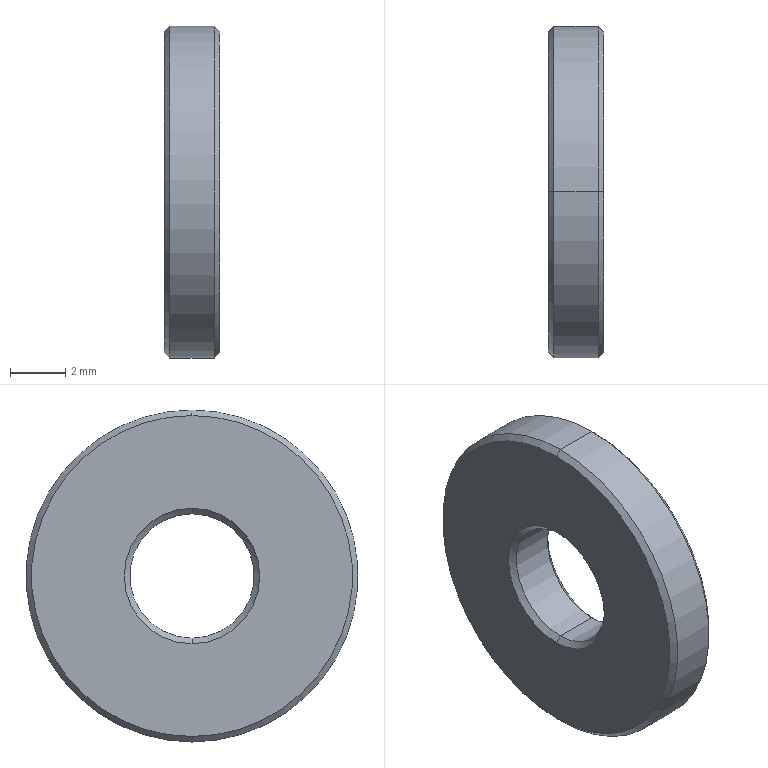Part | STEP file | 03-10 Bearing cover plate 2 | 1 solid | 14 faces | box 2 x 12 x 12 mm | volume 192.313 mm3 | cone 8 | cylinder 4 | plane 2 | commonest cylinder face diameters 4.5 x2 12 x2
STEP:
#1=CARTESIAN_POINT('',(0.,0.,0.));
#2=DIRECTION('',(0.,0.,1.));
#3=DIRECTION('',(1.,0.,0.));
#4=AXIS2_PLACEMENT_3D('',#1,#2,#3);
#5=CARTESIAN_POINT('',(1.8,0.,-2.25));
#6=VERTEX_POINT('',#5);
#7=CARTESIAN_POINT('',(2.,0.,-2.45));
#8=VERTEX_POINT('',#7);
#9=CARTESIAN_POINT('',(1.8,0.,-2.25));
#10=DIRECTION('',(0.7071,0.,-0.7071));
#11=VECTOR('',#10,1.);
#12=LINE('',#9,#11);
#13=CARTESIAN_POINT('',(1.8,0.,0.));
#14=DIRECTION('',(1.,0.,0.));
#15=DIRECTION('',(0.,0.,-1.));
#16=AXIS2_PLACEMENT_3D('',#13,#14,#15);
#17=CONICAL_SURFACE('',#16,2.25,0.7854);
#18=CARTESIAN_POINT('',(6.283,0.));
#19=DIRECTION('',(0.,1.));
#20=VECTOR('',#19,1.);
#21=LINE('',#18,#20);
#22=(GEOMETRIC_REPRESENTATION_CONTEXT(2)PARAMETRIC_REPRESENTATION_CONTEXT()REPRESENTATION_CONTEXT('',''));
#23=DEFINITIONAL_REPRESENTATION('',(#21),#22);
#24=PCURVE('',#17,#23);
#25=CARTESIAN_POINT('',(1.8,0.,0.));
#26=DIRECTION('',(1.,0.,0.));
#27=DIRECTION('',(0.,0.,-1.));
#28=AXIS2_PLACEMENT_3D('',#25,#26,#27);
#29=CONICAL_SURFACE('',#28,2.25,0.7854);
#30=CARTESIAN_POINT('',(0.,0.));
#31=DIRECTION('',(0.,1.));
#32=VECTOR('',#31,1.);
#33=LINE('',#30,#32);
#34=(GEOMETRIC_REPRESENTATION_CONTEXT(2)PARAMETRIC_REPRESENTATION_CONTEXT()REPRESENTATION_CONTEXT('',''));
#35=DEFINITIONAL_REPRESENTATION('',(#33),#34);
#36=PCURVE('',#29,#35);
#37=SURFACE_CURVE('',#12,(#24,#36),.PCURVE_S1.);
#38=EDGE_CURVE('',#6,#8,#37,.T.);
#39=ORIENTED_EDGE('',*,*,#38,.T.);
#40=CARTESIAN_POINT('',(2.,0.,2.45));
#41=VERTEX_POINT('',#40);
#42=CARTESIAN_POINT('',(2.,0.,0.));
#43=DIRECTION('',(1.,0.,0.));
#44=DIRECTION('',(0.,0.,-1.));
#45=AXIS2_PLACEMENT_3D('',#42,#43,#44);
#46=CIRCLE('',#45,2.45);
#47=CARTESIAN_POINT('',(0.,0.2));
#48=DIRECTION('',(1.,0.));
#49=VECTOR('',#48,1.);
#50=LINE('',#47,#49);
#51=(GEOMETRIC_REPRESENTATION_CONTEXT(2)PARAMETRIC_REPRESENTATION_CONTEXT()REPRESENTATION_CONTEXT('',''));
#52=DEFINITIONAL_REPRESENTATION('',(#50),#51);
#53=PCURVE('',#17,#52);
#54=CARTESIAN_POINT('',(2.,-5.87,5.87));
#55=DIRECTION('',(1.,0.,0.));
#56=DIRECTION('',(0.,0.,-1.));
#57=AXIS2_PLACEMENT_3D('',#54,#55,#56);
#58=PLANE('',#57);
#59=CARTESIAN_POINT('',(5.87,5.87));
#60=DIRECTION('',(1.,0.));
#61=AXIS2_PLACEMENT_2D('',#59,#60);
#62=CIRCLE('',#61,2.45);
#63=(GEOMETRIC_REPRESENTATION_CONTEXT(2)PARAMETRIC_REPRESENTATION_CONTEXT()REPRESENTATION_CONTEXT('',''));
#64=DEFINITIONAL_REPRESENTATION('',(#62),#63);
#65=PCURVE('',#58,#64);
#66=SURFACE_CURVE('',#46,(#53,#65),.PCURVE_S1.);
#67=EDGE_CURVE('',#41,#8,#66,.T.);
#68=ORIENTED_EDGE('',*,*,#67,.F.);
#69=CARTESIAN_POINT('',(1.8,0.,2.25));
#70=VERTEX_POINT('',#69);
#71=CARTESIAN_POINT('',(1.8,0.,2.25));
#72=DIRECTION('',(0.7071,0.,0.7071));
#73=VECTOR('',#72,1.);
#74=LINE('',#71,#73);
#75=CARTESIAN_POINT('',(3.142,0.));
#76=DIRECTION('',(0.,1.));
#77=VECTOR('',#76,1.);
#78=LINE('',#75,#77);
#79=(GEOMETRIC_REPRESENTATION_CONTEXT(2)PARAMETRIC_REPRESENTATION_CONTEXT()REPRESENTATION_CONTEXT('',''));
#80=DEFINITIONAL_REPRESENTATION('',(#78),#79);
#81=PCURVE('',#17,#80);
#82=CARTESIAN_POINT('',(3.142,0.));
#83=DIRECTION('',(0.,1.));
#84=VECTOR('',#83,1.);
#85=LINE('',#82,#84);
#86=(GEOMETRIC_REPRESENTATION_CONTEXT(2)PARAMETRIC_REPRESENTATION_CONTEXT()REPRESENTATION_CONTEXT('',''));
#87=DEFINITIONAL_REPRESENTATION('',(#85),#86);
#88=PCURVE('',#29,#87);
#89=SURFACE_CURVE('',#74,(#81,#88),.PCURVE_S1.);
#90=EDGE_CURVE('',#70,#41,#89,.T.);
#91=ORIENTED_EDGE('',*,*,#90,.F.);
#92=CARTESIAN_POINT('',(1.8,0.,0.));
#93=DIRECTION('',(-1.,0.,0.));
#94=DIRECTION('',(0.,0.,-1.));
#95=AXIS2_PLACEMENT_3D('',#92,#93,#94);
#96=CIRCLE('',#95,2.25);
#97=CARTESIAN_POINT('',(6.283,0.));
#98=DIRECTION('',(-1.,0.));
#99=VECTOR('',#98,1.);
#100=LINE('',#97,#99);
#101=(GEOMETRIC_REPRESENTATION_CONTEXT(2)PARAMETRIC_REPRESENTATION_CONTEXT()REPRESENTATION_CONTEXT('',''));
#102=DEFINITIONAL_REPRESENTATION('',(#100),#101);
#103=PCURVE('',#17,#102);
#104=CARTESIAN_POINT('',(1.8,0.,0.));
#105=DIRECTION('',(-1.,0.,0.));
#106=DIRECTION('',(0.,0.,1.));
#107=AXIS2_PLACEMENT_3D('',#104,#105,#106);
#108=CYLINDRICAL_SURFACE('',#107,2.25);
#109=CARTESIAN_POINT('',(3.142,0.));
#110=DIRECTION('',(1.,0.));
#111=VECTOR('',#110,1.);
#112=LINE('',#109,#111);
#113=(GEOMETRIC_REPRESENTATION_CONTEXT(2)PARAMETRIC_REPRESENTATION_CONTEXT()REPRESENTATION_CONTEXT('',''));
#114=DEFINITIONAL_REPRESENTATION('',(#112),#113);
#115=PCURVE('',#108,#114);
#116=SURFACE_CURVE('',#96,(#103,#115),.PCURVE_S1.);
#117=EDGE_CURVE('',#6,#70,#116,.T.);
#118=ORIENTED_EDGE('',*,*,#117,.F.);
#119=EDGE_LOOP('',(#39,#68,#91,#118));
#120=FACE_BOUND('',#119,.F.);
#121=ADVANCED_FACE('',(#120),#17,.F.);
#122=CARTESIAN_POINT('',(0.2,0.,2.25));
#123=VERTEX_POINT('',#122);
#124=CARTESIAN_POINT('',(1.8,0.,2.25));
#125=DIRECTION('',(-1.,0.,0.));
#126=VECTOR('',#125,1.);
#127=LINE('',#124,#126);
#128=CARTESIAN_POINT('',(6.283,0.));
#129=DIRECTION('',(0.,1.));
#130=VECTOR('',#129,1.);
#131=LINE('',#128,#130);
#132=(GEOMETRIC_REPRESENTATION_CONTEXT(2)PARAMETRIC_REPRESENTATION_CONTEXT()REPRESENTATION_CONTEXT('',''));
#133=DEFINITIONAL_REPRESENTATION('',(#131),#132);
#134=PCURVE('',#108,#133);
#135=CARTESIAN_POINT('',(1.8,0.,0.));
#136=DIRECTION('',(-1.,0.,0.));
#137=DIRECTION('',(0.,0.,1.));
#138=AXIS2_PLACEMENT_3D('',#135,#136,#137);
#139=CYLINDRICAL_SURFACE('',#138,2.25);
#140=CARTESIAN_POINT('',(0.,0.));
#141=DIRECTION('',(0.,1.));
#142=VECTOR('',#141,1.);
#143=LINE('',#140,#142);
#144=(GEOMETRIC_REPRESENTATION_CONTEXT(2)PARAMETRIC_REPRESENTATION_CONTEXT()REPRESENTATION_CONTEXT('',''));
#145=DEFINITIONAL_REPRESENTATION('',(#143),#144);
#146=PCURVE('',#139,#145);
#147=SURFACE_CURVE('',#127,(#134,#146),.PCURVE_S1.);
#148=EDGE_CURVE('',#70,#123,#147,.T.);
#149=ORIENTED_EDGE('',*,*,#148,.T.);
#150=CARTESIAN_POINT('',(0.2,0.,-2.25));
#151=VERTEX_POINT('',#150);
#152=CARTESIAN_POINT('',(0.2,0.,0.));
#153=DIRECTION('',(-1.,0.,0.));
#154=DIRECTION('',(0.,0.,1.));
#155=AXIS2_PLACEMENT_3D('',#152,#153,#154);
#156=CIRCLE('',#155,2.25);
#157=CARTESIAN_POINT('',(0.,1.6));
#158=DIRECTION('',(1.,0.));
#159=VECTOR('',#158,1.);
#160=LINE('',#157,#159);
#161=(GEOMETRIC_REPRESENTATION_CONTEXT(2)PARAMETRIC_REPRESENTATION_CONTEXT()REPRESENTATION_CONTEXT('',''));
#162=DEFINITIONAL_REPRESENTATION('',(#160),#161);
#163=PCURVE('',#108,#162);
#164=CARTESIAN_POINT('',(0.2,0.,0.));
#165=DIRECTION('',(-1.,0.,0.));
#166=DIRECTION('',(0.,0.,1.));
#167=AXIS2_PLACEMENT_3D('',#164,#165,#166);
#168=CONICAL_SURFACE('',#167,2.25,0.7854);
#169=CARTESIAN_POINT('',(0.,0.));
#170=DIRECTION('',(1.,0.));
#171=VECTOR('',#170,1.);
#172=LINE('',#169,#171);
#173=(GEOMETRIC_REPRESENTATION_CONTEXT(2)PARAMETRIC_REPRESENTATION_CONTEXT()REPRESENTATION_CONTEXT('',''));
#174=DEFINITIONAL_REPRESENTATION('',(#172),#173);
#175=PCURVE('',#168,#174);
#176=SURFACE_CURVE('',#156,(#163,#175),.PCURVE_S1.);
#177=EDGE_CURVE('',#151,#123,#176,.T.);
#178=ORIENTED_EDGE('',*,*,#177,.F.);
#179=CARTESIAN_POINT('',(1.8,0.,-2.25));
#180=DIRECTION('',(-1.,0.,0.));
#181=VECTOR('',#180,1.);
#182=LINE('',#179,#181);
#183=CARTESIAN_POINT('',(3.142,0.));
#184=DIRECTION('',(0.,1.));
#185=VECTOR('',#184,1.);
#186=LINE('',#183,#185);
#187=(GEOMETRIC_REPRESENTATION_CONTEXT(2)PARAMETRIC_REPRESENTATION_CONTEXT()REPRESENTATION_CONTEXT('',''));
#188=DEFINITIONAL_REPRESENTATION('',(#186),#187);
#189=PCURVE('',#108,#188);
#190=CARTESIAN_POINT('',(3.142,0.));
#191=DIRECTION('',(0.,1.));
#192=VECTOR('',#191,1.);
#193=LINE('',#190,#192);
#194=(GEOMETRIC_REPRESENTATION_CONTEXT(2)PARAMETRIC_REPRESENTATION_CONTEXT()REPRESENTATION_CONTEXT('',''));
#195=DEFINITIONAL_REPRESENTATION('',(#193),#194);
#196=PCURVE('',#139,#195);
#197=SURFACE_CURVE('',#182,(#189,#196),.PCURVE_S1.);
#198=EDGE_CURVE('',#6,#151,#197,.T.);
#199=ORIENTED_EDGE('',*,*,#198,.F.);
#200=ORIENTED_EDGE('',*,*,#117,.T.);
#201=EDGE_LOOP('',(#149,#178,#199,#200));
#202=FACE_BOUND('',#201,.F.);
#203=ADVANCED_FACE('',(#202),#108,.F.);
#204=CARTESIAN_POINT('',(2.,0.,-5.8));
#205=VERTEX_POINT('',#204);
#206=CARTESIAN_POINT('',(2.,0.,5.8));
#207=VERTEX_POINT('',#206);
#208=CARTESIAN_POINT('',(2.,0.,0.));
#209=DIRECTION('',(1.,0.,0.));
#210=DIRECTION('',(0.,0.,1.));
#211=AXIS2_PLACEMENT_3D('',#208,#209,#210);
#212=CIRCLE('',#211,5.8);
#213=CARTESIAN_POINT('',(2.,0.,0.));
#214=DIRECTION('',(-1.,0.,0.));
#215=DIRECTION('',(0.,0.,1.));
#216=AXIS2_PLACEMENT_3D('',#213,#214,#215);
#217=CONICAL_SURFACE('',#216,5.8,0.7854);
#218=CARTESIAN_POINT('',(6.283,0.));
#219=DIRECTION('',(-1.,0.));
#220=VECTOR('',#219,1.);
#221=LINE('',#218,#220);
#222=(GEOMETRIC_REPRESENTATION_CONTEXT(2)PARAMETRIC_REPRESENTATION_CONTEXT()REPRESENTATION_CONTEXT('',''));
#223=DEFINITIONAL_REPRESENTATION('',(#221),#222);
#224=PCURVE('',#217,#223);
#225=CARTESIAN_POINT('',(5.87,5.87));
#226=DIRECTION('',(-1.,0.));
#227=AXIS2_PLACEMENT_2D('',#225,#226);
#228=CIRCLE('',#227,5.8);
#229=(GEOMETRIC_REPRESENTATION_CONTEXT(2)PARAMETRIC_REPRESENTATION_CONTEXT()REPRESENTATION_CONTEXT('',''));
#230=DEFINITIONAL_REPRESENTATION('',(#228),#229);
#231=PCURVE('',#58,#230);
#232=SURFACE_CURVE('',#212,(#224,#231),.PCURVE_S1.);
#233=EDGE_CURVE('',#205,#207,#232,.T.);
#234=ORIENTED_EDGE('',*,*,#233,.F.);
#235=CARTESIAN_POINT('',(1.8,0.,-6.));
#236=VERTEX_POINT('',#235);
#237=CARTESIAN_POINT('',(2.,0.,-5.8));
#238=DIRECTION('',(-0.7071,0.,-0.7071));
#239=VECTOR('',#238,1.);
#240=LINE('',#237,#239);
#241=CARTESIAN_POINT('',(3.142,0.));
#242=DIRECTION('',(0.,1.));
#243=VECTOR('',#242,1.);
#244=LINE('',#241,#243);
#245=(GEOMETRIC_REPRESENTATION_CONTEXT(2)PARAMETRIC_REPRESENTATION_CONTEXT()REPRESENTATION_CONTEXT('',''));
#246=DEFINITIONAL_REPRESENTATION('',(#244),#245);
#247=PCURVE('',#217,#246);
#248=CARTESIAN_POINT('',(2.,0.,0.));
#249=DIRECTION('',(-1.,0.,0.));
#250=DIRECTION('',(0.,0.,1.));
#251=AXIS2_PLACEMENT_3D('',#248,#249,#250);
#252=CONICAL_SURFACE('',#251,5.8,0.7854);
#253=CARTESIAN_POINT('',(3.142,0.));
#254=DIRECTION('',(0.,1.));
#255=VECTOR('',#254,1.);
#256=LINE('',#253,#255);
#257=(GEOMETRIC_REPRESENTATION_CONTEXT(2)PARAMETRIC_REPRESENTATION_CONTEXT()REPRESENTATION_CONTEXT('',''));
#258=DEFINITIONAL_REPRESENTATION('',(#256),#257);
#259=PCURVE('',#252,#258);
#260=SURFACE_CURVE('',#240,(#247,#259),.PCURVE_S1.);
#261=EDGE_CURVE('',#205,#236,#260,.T.);
#262=ORIENTED_EDGE('',*,*,#261,.T.);
#263=CARTESIAN_POINT('',(1.8,0.,6.));
#264=VERTEX_POINT('',#263);
#265=CARTESIAN_POINT('',(1.8,0.,0.));
#266=DIRECTION('',(-1.,0.,0.));
#267=DIRECTION('',(0.,0.,1.));
#268=AXIS2_PLACEMENT_3D('',#265,#266,#267);
#269=CIRCLE('',#268,6.);
#270=CARTESIAN_POINT('',(0.,0.2));
#271=DIRECTION('',(1.,0.));
#272=VECTOR('',#271,1.);
#273=LINE('',#270,#272);
#274=(GEOMETRIC_REPRESENTATION_CONTEXT(2)PARAMETRIC_REPRESENTATION_CONTEXT()REPRESENTATION_CONTEXT('',''));
#275=DEFINITIONAL_REPRESENTATION('',(#273),#274);
#276=PCURVE('',#217,#275);
#277=CARTESIAN_POINT('',(1.8,0.,0.));
#278=DIRECTION('',(-1.,0.,0.));
#279=DIRECTION('',(0.,0.,1.));
#280=AXIS2_PLACEMENT_3D('',#277,#278,#279);
#281=CYLINDRICAL_SURFACE('',#280,6.);
#282=CARTESIAN_POINT('',(0.,0.));
#283=DIRECTION('',(1.,0.));
#284=VECTOR('',#283,1.);
#285=LINE('',#282,#284);
#286=(GEOMETRIC_REPRESENTATION_CONTEXT(2)PARAMETRIC_REPRESENTATION_CONTEXT()REPRESENTATION_CONTEXT('',''));
#287=DEFINITIONAL_REPRESENTATION('',(#285),#286);
#288=PCURVE('',#281,#287);
#289=SURFACE_CURVE('',#269,(#276,#288),.PCURVE_S1.);
#290=EDGE_CURVE('',#264,#236,#289,.T.);
#291=ORIENTED_EDGE('',*,*,#290,.F.);
#292=CARTESIAN_POINT('',(2.,0.,5.8));
#293=DIRECTION('',(-0.7071,0.,0.7071));
#294=VECTOR('',#293,1.);
#295=LINE('',#292,#294);
#296=CARTESIAN_POINT('',(0.,0.));
#297=DIRECTION('',(0.,1.));
#298=VECTOR('',#297,1.);
#299=LINE('',#296,#298);
#300=(GEOMETRIC_REPRESENTATION_CONTEXT(2)PARAMETRIC_REPRESENTATION_CONTEXT()REPRESENTATION_CONTEXT('',''));
#301=DEFINITIONAL_REPRESENTATION('',(#299),#300);
#302=PCURVE('',#217,#301);
#303=CARTESIAN_POINT('',(6.283,0.));
#304=DIRECTION('',(0.,1.));
#305=VECTOR('',#304,1.);
#306=LINE('',#303,#305);
#307=(GEOMETRIC_REPRESENTATION_CONTEXT(2)PARAMETRIC_REPRESENTATION_CONTEXT()REPRESENTATION_CONTEXT('',''));
#308=DEFINITIONAL_REPRESENTATION('',(#306),#307);
#309=PCURVE('',#252,#308);
#310=SURFACE_CURVE('',#295,(#302,#309),.PCURVE_S1.);
#311=EDGE_CURVE('',#207,#264,#310,.T.);
#312=ORIENTED_EDGE('',*,*,#311,.F.);
#313=EDGE_LOOP('',(#234,#262,#291,#312));
#314=FACE_BOUND('',#313,.T.);
#315=ADVANCED_FACE('',(#314),#217,.T.);
#316=CARTESIAN_POINT('',(0.,0.,2.45));
#317=VERTEX_POINT('',#316);
#318=CARTESIAN_POINT('',(0.2,0.,2.25));
#319=DIRECTION('',(-0.7071,0.,0.7071));
#320=VECTOR('',#319,1.);
#321=LINE('',#318,#320);
#322=CARTESIAN_POINT('',(6.283,0.));
#323=DIRECTION('',(0.,1.));
#324=VECTOR('',#323,1.);
#325=LINE('',#322,#324);
#326=(GEOMETRIC_REPRESENTATION_CONTEXT(2)PARAMETRIC_REPRESENTATION_CONTEXT()REPRESENTATION_CONTEXT('',''));
#327=DEFINITIONAL_REPRESENTATION('',(#325),#326);
#328=PCURVE('',#168,#327);
#329=CARTESIAN_POINT('',(0.2,0.,0.));
#330=DIRECTION('',(-1.,0.,0.));
#331=DIRECTION('',(0.,0.,1.));
#332=AXIS2_PLACEMENT_3D('',#329,#330,#331);
#333=CONICAL_SURFACE('',#332,2.25,0.7854);
#334=CARTESIAN_POINT('',(0.,0.));
#335=DIRECTION('',(0.,1.));
#336=VECTOR('',#335,1.);
#337=LINE('',#334,#336);
#338=(GEOMETRIC_REPRESENTATION_CONTEXT(2)PARAMETRIC_REPRESENTATION_CONTEXT()REPRESENTATION_CONTEXT('',''));
#339=DEFINITIONAL_REPRESENTATION('',(#337),#338);
#340=PCURVE('',#333,#339);
#341=SURFACE_CURVE('',#321,(#328,#340),.PCURVE_S1.);
#342=EDGE_CURVE('',#123,#317,#341,.T.);
#343=ORIENTED_EDGE('',*,*,#342,.T.);
#344=CARTESIAN_POINT('',(0.,0.,-2.45));
#345=VERTEX_POINT('',#344);
#346=CARTESIAN_POINT('',(0.,0.,0.));
#347=DIRECTION('',(-1.,0.,0.));
#348=DIRECTION('',(0.,0.,1.));
#349=AXIS2_PLACEMENT_3D('',#346,#347,#348);
#350=CIRCLE('',#349,2.45);
#351=CARTESIAN_POINT('',(0.,0.2));
#352=DIRECTION('',(1.,0.));
#353=VECTOR('',#352,1.);
#354=LINE('',#351,#353);
#355=(GEOMETRIC_REPRESENTATION_CONTEXT(2)PARAMETRIC_REPRESENTATION_CONTEXT()REPRESENTATION_CONTEXT('',''));
#356=DEFINITIONAL_REPRESENTATION('',(#354),#355);
#357=PCURVE('',#168,#356);
#358=CARTESIAN_POINT('',(0.,-5.87,5.87));
#359=DIRECTION('',(1.,0.,0.));
#360=DIRECTION('',(0.,0.,-1.));
#361=AXIS2_PLACEMENT_3D('',#358,#359,#360);
#362=PLANE('',#361);
#363=CARTESIAN_POINT('',(3.42,5.87));
#364=CARTESIAN_POINT('',(3.42,10.113));
#365=CARTESIAN_POINT('',(7.095,7.991));
#366=CARTESIAN_POINT('',(10.77,5.87));
#367=CARTESIAN_POINT('',(7.095,3.748));
#368=CARTESIAN_POINT('',(3.42,1.626));
#369=CARTESIAN_POINT('',(3.42,5.87));
#370=(BOUNDED_CURVE()B_SPLINE_CURVE(2,(#363,#364,#365,#366,#367,#368,#369),.UNSPECIFIED.,.T.,.F.)B_SPLINE_CURVE_WITH_KNOTS((1,2,2,2,2,1),(-2.094,0.,2.094,4.189,6.283,8.378),.UNSPECIFIED.)CURVE()GEOMETRIC_REPRESENTATION_ITEM()RATIONAL_B_SPLINE_CURVE((1.,0.5,1.,0.5,1.,0.5,1.))REPRESENTATION_ITEM(''));
#371=(GEOMETRIC_REPRESENTATION_CONTEXT(2)PARAMETRIC_REPRESENTATION_CONTEXT()REPRESENTATION_CONTEXT('',''));
#372=DEFINITIONAL_REPRESENTATION('',(#370),#371);
#373=PCURVE('',#362,#372);
#374=SURFACE_CURVE('',#350,(#357,#373),.PCURVE_S1.);
#375=EDGE_CURVE('',#345,#317,#374,.T.);
#376=ORIENTED_EDGE('',*,*,#375,.F.);
#377=CARTESIAN_POINT('',(0.2,0.,-2.25));
#378=DIRECTION('',(-0.7071,0.,-0.7071));
#379=VECTOR('',#378,1.);
#380=LINE('',#377,#379);
#381=CARTESIAN_POINT('',(3.142,0.));
#382=DIRECTION('',(0.,1.));
#383=VECTOR('',#382,1.);
#384=LINE('',#381,#383);
#385=(GEOMETRIC_REPRESENTATION_CONTEXT(2)PARAMETRIC_REPRESENTATION_CONTEXT()REPRESENTATION_CONTEXT('',''));
#386=DEFINITIONAL_REPRESENTATION('',(#384),#385);
#387=PCURVE('',#168,#386);
#388=CARTESIAN_POINT('',(3.142,0.));
#389=DIRECTION('',(0.,1.));
#390=VECTOR('',#389,1.);
#391=LINE('',#388,#390);
#392=(GEOMETRIC_REPRESENTATION_CONTEXT(2)PARAMETRIC_REPRESENTATION_CONTEXT()REPRESENTATION_CONTEXT('',''));
#393=DEFINITIONAL_REPRESENTATION('',(#391),#392);
#394=PCURVE('',#333,#393);
#395=SURFACE_CURVE('',#380,(#387,#394),.PCURVE_S1.);
#396=EDGE_CURVE('',#151,#345,#395,.T.);
#397=ORIENTED_EDGE('',*,*,#396,.F.);
#398=ORIENTED_EDGE('',*,*,#177,.T.);
#399=EDGE_LOOP('',(#343,#376,#397,#398));
#400=FACE_BOUND('',#399,.F.);
#401=ADVANCED_FACE('',(#400),#168,.F.);
#402=ORIENTED_EDGE('',*,*,#290,.T.);
#403=CARTESIAN_POINT('',(0.2,0.,-6.));
#404=VERTEX_POINT('',#403);
#405=CARTESIAN_POINT('',(1.8,0.,-6.));
#406=DIRECTION('',(-1.,0.,0.));
#407=VECTOR('',#406,1.);
#408=LINE('',#405,#407);
#409=CARTESIAN_POINT('',(3.142,0.));
#410=DIRECTION('',(0.,1.));
#411=VECTOR('',#410,1.);
#412=LINE('',#409,#411);
#413=(GEOMETRIC_REPRESENTATION_CONTEXT(2)PARAMETRIC_REPRESENTATION_CONTEXT()REPRESENTATION_CONTEXT('',''));
#414=DEFINITIONAL_REPRESENTATION('',(#412),#413);
#415=PCURVE('',#281,#414);
#416=CARTESIAN_POINT('',(1.8,0.,0.));
#417=DIRECTION('',(-1.,0.,0.));
#418=DIRECTION('',(0.,0.,1.));
#419=AXIS2_PLACEMENT_3D('',#416,#417,#418);
#420=CYLINDRICAL_SURFACE('',#419,6.);
#421=CARTESIAN_POINT('',(3.142,0.));
#422=DIRECTION('',(0.,1.));
#423=VECTOR('',#422,1.);
#424=LINE('',#421,#423);
#425=(GEOMETRIC_REPRESENTATION_CONTEXT(2)PARAMETRIC_REPRESENTATION_CONTEXT()REPRESENTATION_CONTEXT('',''));
#426=DEFINITIONAL_REPRESENTATION('',(#424),#425);
#427=PCURVE('',#420,#426);
#428=SURFACE_CURVE('',#408,(#415,#427),.PCURVE_S1.);
#429=EDGE_CURVE('',#236,#404,#428,.T.);
#430=ORIENTED_EDGE('',*,*,#429,.T.);
#431=CARTESIAN_POINT('',(0.2,0.,6.));
#432=VERTEX_POINT('',#431);
#433=CARTESIAN_POINT('',(0.2,0.,0.));
#434=DIRECTION('',(-1.,0.,0.));
#435=DIRECTION('',(0.,0.,1.));
#436=AXIS2_PLACEMENT_3D('',#433,#434,#435);
#437=CIRCLE('',#436,6.);
#438=CARTESIAN_POINT('',(0.,1.6));
#439=DIRECTION('',(1.,0.));
#440=VECTOR('',#439,1.);
#441=LINE('',#438,#440);
#442=(GEOMETRIC_REPRESENTATION_CONTEXT(2)PARAMETRIC_REPRESENTATION_CONTEXT()REPRESENTATION_CONTEXT('',''));
#443=DEFINITIONAL_REPRESENTATION('',(#441),#442);
#444=PCURVE('',#281,#443);
#445=CARTESIAN_POINT('',(0.,0.,0.));
#446=DIRECTION('',(1.,0.,0.));
#447=DIRECTION('',(0.,0.,-1.));
#448=AXIS2_PLACEMENT_3D('',#445,#446,#447);
#449=CONICAL_SURFACE('',#448,5.8,0.7854);
#450=CARTESIAN_POINT('',(3.142,0.2));
#451=DIRECTION('',(-1.,0.));
#452=VECTOR('',#451,1.);
#453=LINE('',#450,#452);
#454=(GEOMETRIC_REPRESENTATION_CONTEXT(2)PARAMETRIC_REPRESENTATION_CONTEXT()REPRESENTATION_CONTEXT('',''));
#455=DEFINITIONAL_REPRESENTATION('',(#453),#454);
#456=PCURVE('',#449,#455);
#457=SURFACE_CURVE('',#437,(#444,#456),.PCURVE_S1.);
#458=EDGE_CURVE('',#432,#404,#457,.T.);
#459=ORIENTED_EDGE('',*,*,#458,.F.);
#460=CARTESIAN_POINT('',(1.8,0.,6.));
#461=DIRECTION('',(-1.,0.,0.));
#462=VECTOR('',#461,1.);
#463=LINE('',#460,#462);
#464=CARTESIAN_POINT('',(0.,0.));
#465=DIRECTION('',(0.,1.));
#466=VECTOR('',#465,1.);
#467=LINE('',#464,#466);
#468=(GEOMETRIC_REPRESENTATION_CONTEXT(2)PARAMETRIC_REPRESENTATION_CONTEXT()REPRESENTATION_CONTEXT('',''));
#469=DEFINITIONAL_REPRESENTATION('',(#467),#468);
#470=PCURVE('',#281,#469);
#471=CARTESIAN_POINT('',(6.283,0.));
#472=DIRECTION('',(0.,1.));
#473=VECTOR('',#472,1.);
#474=LINE('',#471,#473);
#475=(GEOMETRIC_REPRESENTATION_CONTEXT(2)PARAMETRIC_REPRESENTATION_CONTEXT()REPRESENTATION_CONTEXT('',''));
#476=DEFINITIONAL_REPRESENTATION('',(#474),#475);
#477=PCURVE('',#420,#476);
#478=SURFACE_CURVE('',#463,(#470,#477),.PCURVE_S1.);
#479=EDGE_CURVE('',#264,#432,#478,.T.);
#480=ORIENTED_EDGE('',*,*,#479,.F.);
#481=EDGE_LOOP('',(#402,#430,#459,#480));
#482=FACE_BOUND('',#481,.T.);
#483=ADVANCED_FACE('',(#482),#281,.T.);
#484=CARTESIAN_POINT('',(0.,0.,-5.8));
#485=VERTEX_POINT('',#484);
#486=CARTESIAN_POINT('',(0.,0.,5.8));
#487=VERTEX_POINT('',#486);
#488=CARTESIAN_POINT('',(0.,0.,0.));
#489=DIRECTION('',(1.,0.,0.));
#490=DIRECTION('',(0.,0.,-1.));
#491=AXIS2_PLACEMENT_3D('',#488,#489,#490);
#492=CIRCLE('',#491,5.8);
#493=CARTESIAN_POINT('',(0.,0.));
#494=DIRECTION('',(1.,0.));
#495=VECTOR('',#494,1.);
#496=LINE('',#493,#495);
#497=(GEOMETRIC_REPRESENTATION_CONTEXT(2)PARAMETRIC_REPRESENTATION_CONTEXT()REPRESENTATION_CONTEXT('',''));
#498=DEFINITIONAL_REPRESENTATION('',(#496),#497);
#499=PCURVE('',#449,#498);
#500=CARTESIAN_POINT('',(5.87,5.87));
#501=DIRECTION('',(1.,0.));
#502=AXIS2_PLACEMENT_2D('',#500,#501);
#503=CIRCLE('',#502,5.8);
#504=(GEOMETRIC_REPRESENTATION_CONTEXT(2)PARAMETRIC_REPRESENTATION_CONTEXT()REPRESENTATION_CONTEXT('',''));
#505=DEFINITIONAL_REPRESENTATION('',(#503),#504);
#506=PCURVE('',#362,#505);
#507=SURFACE_CURVE('',#492,(#499,#506),.PCURVE_S1.);
#508=EDGE_CURVE('',#485,#487,#507,.T.);
#509=ORIENTED_EDGE('',*,*,#508,.T.);
#510=CARTESIAN_POINT('',(0.,0.,5.8));
#511=DIRECTION('',(0.7071,0.,0.7071));
#512=VECTOR('',#511,1.);
#513=LINE('',#510,#512);
#514=CARTESIAN_POINT('',(3.142,0.));
#515=DIRECTION('',(0.,1.));
#516=VECTOR('',#515,1.);
#517=LINE('',#514,#516);
#518=(GEOMETRIC_REPRESENTATION_CONTEXT(2)PARAMETRIC_REPRESENTATION_CONTEXT()REPRESENTATION_CONTEXT('',''));
#519=DEFINITIONAL_REPRESENTATION('',(#517),#518);
#520=PCURVE('',#449,#519);
#521=CARTESIAN_POINT('',(0.,0.,0.));
#522=DIRECTION('',(1.,0.,0.));
#523=DIRECTION('',(0.,0.,-1.));
#524=AXIS2_PLACEMENT_3D('',#521,#522,#523);
#525=CONICAL_SURFACE('',#524,5.8,0.7854);
#526=CARTESIAN_POINT('',(3.142,0.));
#527=DIRECTION('',(0.,1.));
#528=VECTOR('',#527,1.);
#529=LINE('',#526,#528);
#530=(GEOMETRIC_REPRESENTATION_CONTEXT(2)PARAMETRIC_REPRESENTATION_CONTEXT()REPRESENTATION_CONTEXT('',''));
#531=DEFINITIONAL_REPRESENTATION('',(#529),#530);
#532=PCURVE('',#525,#531);
#533=SURFACE_CURVE('',#513,(#520,#532),.PCURVE_S1.);
#534=EDGE_CURVE('',#487,#432,#533,.T.);
#535=ORIENTED_EDGE('',*,*,#534,.T.);
#536=ORIENTED_EDGE('',*,*,#458,.T.);
#537=CARTESIAN_POINT('',(0.,0.,-5.8));
#538=DIRECTION('',(0.7071,0.,-0.7071));
#539=VECTOR('',#538,1.);
#540=LINE('',#537,#539);
#541=CARTESIAN_POINT('',(0.,0.));
#542=DIRECTION('',(0.,1.));
#543=VECTOR('',#542,1.);
#544=LINE('',#541,#543);
#545=(GEOMETRIC_REPRESENTATION_CONTEXT(2)PARAMETRIC_REPRESENTATION_CONTEXT()REPRESENTATION_CONTEXT('',''));
#546=DEFINITIONAL_REPRESENTATION('',(#544),#545);
#547=PCURVE('',#449,#546);
#548=CARTESIAN_POINT('',(6.283,0.));
#549=DIRECTION('',(0.,1.));
#550=VECTOR('',#549,1.);
#551=LINE('',#548,#550);
#552=(GEOMETRIC_REPRESENTATION_CONTEXT(2)PARAMETRIC_REPRESENTATION_CONTEXT()REPRESENTATION_CONTEXT('',''));
#553=DEFINITIONAL_REPRESENTATION('',(#551),#552);
#554=PCURVE('',#525,#553);
#555=SURFACE_CURVE('',#540,(#547,#554),.PCURVE_S1.);
#556=EDGE_CURVE('',#485,#404,#555,.T.);
#557=ORIENTED_EDGE('',*,*,#556,.F.);
#558=EDGE_LOOP('',(#509,#535,#536,#557));
#559=FACE_BOUND('',#558,.T.);
#560=ADVANCED_FACE('',(#559),#449,.T.);
#561=CARTESIAN_POINT('',(2.,0.,0.));
#562=DIRECTION('',(1.,0.,0.));
#563=DIRECTION('',(0.,0.,-1.));
#564=AXIS2_PLACEMENT_3D('',#561,#562,#563);
#565=CIRCLE('',#564,2.45);
#566=CARTESIAN_POINT('',(0.,0.2));
#567=DIRECTION('',(1.,0.));
#568=VECTOR('',#567,1.);
#569=LINE('',#566,#568);
#570=(GEOMETRIC_REPRESENTATION_CONTEXT(2)PARAMETRIC_REPRESENTATION_CONTEXT()REPRESENTATION_CONTEXT('',''));
#571=DEFINITIONAL_REPRESENTATION('',(#569),#570);
#572=PCURVE('',#29,#571);
#573=CARTESIAN_POINT('',(5.87,5.87));
#574=DIRECTION('',(1.,0.));
#575=AXIS2_PLACEMENT_2D('',#573,#574);
#576=CIRCLE('',#575,2.45);
#577=(GEOMETRIC_REPRESENTATION_CONTEXT(2)PARAMETRIC_REPRESENTATION_CONTEXT()REPRESENTATION_CONTEXT('',''));
#578=DEFINITIONAL_REPRESENTATION('',(#576),#577);
#579=PCURVE('',#58,#578);
#580=SURFACE_CURVE('',#565,(#572,#579),.PCURVE_S1.);
#581=EDGE_CURVE('',#8,#41,#580,.T.);
#582=ORIENTED_EDGE('',*,*,#581,.F.);
#583=ORIENTED_EDGE('',*,*,#38,.F.);
#584=CARTESIAN_POINT('',(1.8,0.,0.));
#585=DIRECTION('',(-1.,0.,0.));
#586=DIRECTION('',(0.,0.,-1.));
#587=AXIS2_PLACEMENT_3D('',#584,#585,#586);
#588=CIRCLE('',#587,2.25);
#589=CARTESIAN_POINT('',(6.283,0.));
#590=DIRECTION('',(-1.,0.));
#591=VECTOR('',#590,1.);
#592=LINE('',#589,#591);
#593=(GEOMETRIC_REPRESENTATION_CONTEXT(2)PARAMETRIC_REPRESENTATION_CONTEXT()REPRESENTATION_CONTEXT('',''));
#594=DEFINITIONAL_REPRESENTATION('',(#592),#593);
#595=PCURVE('',#29,#594);
#596=CARTESIAN_POINT('',(-3.142,0.));
#597=DIRECTION('',(1.,0.));
#598=VECTOR('',#597,1.);
#599=LINE('',#596,#598);
#600=(GEOMETRIC_REPRESENTATION_CONTEXT(2)PARAMETRIC_REPRESENTATION_CONTEXT()REPRESENTATION_CONTEXT('',''));
#601=DEFINITIONAL_REPRESENTATION('',(#599),#600);
#602=PCURVE('',#139,#601);
#603=SURFACE_CURVE('',#588,(#595,#602),.PCURVE_S1.);
#604=EDGE_CURVE('',#70,#6,#603,.T.);
#605=ORIENTED_EDGE('',*,*,#604,.F.);
#606=ORIENTED_EDGE('',*,*,#90,.T.);
#607=EDGE_LOOP('',(#582,#583,#605,#606));
#608=FACE_BOUND('',#607,.F.);
#609=ADVANCED_FACE('',(#608),#29,.F.);
#610=ORIENTED_EDGE('',*,*,#581,.F.);
#611=ORIENTED_EDGE('',*,*,#67,.F.);
#612=EDGE_LOOP('',(#610,#611));
#613=FACE_BOUND('',#612,.T.);
#614=CARTESIAN_POINT('',(2.,0.,0.));
#615=DIRECTION('',(1.,0.,0.));
#616=DIRECTION('',(0.,0.,1.));
#617=AXIS2_PLACEMENT_3D('',#614,#615,#616);
#618=CIRCLE('',#617,5.8);
#619=CARTESIAN_POINT('',(5.87,5.87));
#620=DIRECTION('',(-1.,0.));
#621=AXIS2_PLACEMENT_2D('',#619,#620);
#622=CIRCLE('',#621,5.8);
#623=(GEOMETRIC_REPRESENTATION_CONTEXT(2)PARAMETRIC_REPRESENTATION_CONTEXT()REPRESENTATION_CONTEXT('',''));
#624=DEFINITIONAL_REPRESENTATION('',(#622),#623);
#625=PCURVE('',#58,#624);
#626=CARTESIAN_POINT('',(6.283,0.));
#627=DIRECTION('',(-1.,0.));
#628=VECTOR('',#627,1.);
#629=LINE('',#626,#628);
#630=(GEOMETRIC_REPRESENTATION_CONTEXT(2)PARAMETRIC_REPRESENTATION_CONTEXT()REPRESENTATION_CONTEXT('',''));
#631=DEFINITIONAL_REPRESENTATION('',(#629),#630);
#632=PCURVE('',#252,#631);
#633=SURFACE_CURVE('',#618,(#625,#632),.PCURVE_S1.);
#634=EDGE_CURVE('',#207,#205,#633,.T.);
#635=ORIENTED_EDGE('',*,*,#634,.T.);
#636=ORIENTED_EDGE('',*,*,#233,.T.);
#637=EDGE_LOOP('',(#635,#636));
#638=FACE_BOUND('',#637,.T.);
#639=ADVANCED_FACE('',(#613,#638),#58,.T.);
#640=CARTESIAN_POINT('',(0.2,0.,0.));
#641=DIRECTION('',(-1.,0.,0.));
#642=DIRECTION('',(0.,0.,1.));
#643=AXIS2_PLACEMENT_3D('',#640,#641,#642);
#644=CIRCLE('',#643,2.25);
#645=CARTESIAN_POINT('',(0.,1.6));
#646=DIRECTION('',(1.,0.));
#647=VECTOR('',#646,1.);
#648=LINE('',#645,#647);
#649=(GEOMETRIC_REPRESENTATION_CONTEXT(2)PARAMETRIC_REPRESENTATION_CONTEXT()REPRESENTATION_CONTEXT('',''));
#650=DEFINITIONAL_REPRESENTATION('',(#648),#649);
#651=PCURVE('',#139,#650);
#652=CARTESIAN_POINT('',(0.,0.));
#653=DIRECTION('',(1.,0.));
#654=VECTOR('',#653,1.);
#655=LINE('',#652,#654);
#656=(GEOMETRIC_REPRESENTATION_CONTEXT(2)PARAMETRIC_REPRESENTATION_CONTEXT()REPRESENTATION_CONTEXT('',''));
#657=DEFINITIONAL_REPRESENTATION('',(#655),#656);
#658=PCURVE('',#333,#657);
#659=SURFACE_CURVE('',#644,(#651,#658),.PCURVE_S1.);
#660=EDGE_CURVE('',#123,#151,#659,.T.);
#661=ORIENTED_EDGE('',*,*,#660,.F.);
#662=ORIENTED_EDGE('',*,*,#148,.F.);
#663=ORIENTED_EDGE('',*,*,#604,.T.);
#664=ORIENTED_EDGE('',*,*,#198,.T.);
#665=EDGE_LOOP('',(#661,#662,#663,#664));
#666=FACE_BOUND('',#665,.F.);
#667=ADVANCED_FACE('',(#666),#139,.F.);
#668=ORIENTED_EDGE('',*,*,#261,.F.);
#669=ORIENTED_EDGE('',*,*,#634,.F.);
#670=ORIENTED_EDGE('',*,*,#311,.T.);
#671=CARTESIAN_POINT('',(1.8,0.,0.));
#672=DIRECTION('',(-1.,0.,0.));
#673=DIRECTION('',(0.,0.,1.));
#674=AXIS2_PLACEMENT_3D('',#671,#672,#673);
#675=CIRCLE('',#674,6.);
#676=CARTESIAN_POINT('',(0.,0.2));
#677=DIRECTION('',(1.,0.));
#678=VECTOR('',#677,1.);
#679=LINE('',#676,#678);
#680=(GEOMETRIC_REPRESENTATION_CONTEXT(2)PARAMETRIC_REPRESENTATION_CONTEXT()REPRESENTATION_CONTEXT('',''));
#681=DEFINITIONAL_REPRESENTATION('',(#679),#680);
#682=PCURVE('',#252,#681);
#683=CARTESIAN_POINT('',(0.,0.));
#684=DIRECTION('',(1.,0.));
#685=VECTOR('',#684,1.);
#686=LINE('',#683,#685);
#687=(GEOMETRIC_REPRESENTATION_CONTEXT(2)PARAMETRIC_REPRESENTATION_CONTEXT()REPRESENTATION_CONTEXT('',''));
#688=DEFINITIONAL_REPRESENTATION('',(#686),#687);
#689=PCURVE('',#420,#688);
#690=SURFACE_CURVE('',#675,(#682,#689),.PCURVE_S1.);
#691=EDGE_CURVE('',#236,#264,#690,.T.);
#692=ORIENTED_EDGE('',*,*,#691,.F.);
#693=EDGE_LOOP('',(#668,#669,#670,#692));
#694=FACE_BOUND('',#693,.T.);
#695=ADVANCED_FACE('',(#694),#252,.T.);
#696=CARTESIAN_POINT('',(0.,0.,0.));
#697=DIRECTION('',(-1.,0.,0.));
#698=DIRECTION('',(0.,0.,1.));
#699=AXIS2_PLACEMENT_3D('',#696,#697,#698);
#700=CIRCLE('',#699,2.45);
#701=CARTESIAN_POINT('',(0.,0.2));
#702=DIRECTION('',(1.,0.));
#703=VECTOR('',#702,1.);
#704=LINE('',#701,#703);
#705=(GEOMETRIC_REPRESENTATION_CONTEXT(2)PARAMETRIC_REPRESENTATION_CONTEXT()REPRESENTATION_CONTEXT('',''));
#706=DEFINITIONAL_REPRESENTATION('',(#704),#705);
#707=PCURVE('',#333,#706);
#708=CARTESIAN_POINT('',(3.42,5.87));
#709=CARTESIAN_POINT('',(3.42,10.113));
#710=CARTESIAN_POINT('',(7.095,7.991));
#711=CARTESIAN_POINT('',(10.77,5.87));
#712=CARTESIAN_POINT('',(7.095,3.748));
#713=CARTESIAN_POINT('',(3.42,1.626));
#714=CARTESIAN_POINT('',(3.42,5.87));
#715=(BOUNDED_CURVE()B_SPLINE_CURVE(2,(#708,#709,#710,#711,#712,#713,#714),.UNSPECIFIED.,.T.,.F.)B_SPLINE_CURVE_WITH_KNOTS((1,2,2,2,2,1),(-2.094,0.,2.094,4.189,6.283,8.378),.UNSPECIFIED.)CURVE()GEOMETRIC_REPRESENTATION_ITEM()RATIONAL_B_SPLINE_CURVE((1.,0.5,1.,0.5,1.,0.5,1.))REPRESENTATION_ITEM(''));
#716=(GEOMETRIC_REPRESENTATION_CONTEXT(2)PARAMETRIC_REPRESENTATION_CONTEXT()REPRESENTATION_CONTEXT('',''));
#717=DEFINITIONAL_REPRESENTATION('',(#715),#716);
#718=PCURVE('',#362,#717);
#719=SURFACE_CURVE('',#700,(#707,#718),.PCURVE_S1.);
#720=EDGE_CURVE('',#317,#345,#719,.T.);
#721=ORIENTED_EDGE('',*,*,#720,.F.);
#722=ORIENTED_EDGE('',*,*,#342,.F.);
#723=ORIENTED_EDGE('',*,*,#660,.T.);
#724=ORIENTED_EDGE('',*,*,#396,.T.);
#725=EDGE_LOOP('',(#721,#722,#723,#724));
#726=FACE_BOUND('',#725,.F.);
#727=ADVANCED_FACE('',(#726),#333,.F.);
#728=ORIENTED_EDGE('',*,*,#429,.F.);
#729=ORIENTED_EDGE('',*,*,#691,.T.);
#730=ORIENTED_EDGE('',*,*,#479,.T.);
#731=CARTESIAN_POINT('',(0.2,0.,0.));
#732=DIRECTION('',(-1.,0.,0.));
#733=DIRECTION('',(0.,0.,1.));
#734=AXIS2_PLACEMENT_3D('',#731,#732,#733);
#735=CIRCLE('',#734,6.);
#736=CARTESIAN_POINT('',(0.,1.6));
#737=DIRECTION('',(1.,0.));
#738=VECTOR('',#737,1.);
#739=LINE('',#736,#738);
#740=(GEOMETRIC_REPRESENTATION_CONTEXT(2)PARAMETRIC_REPRESENTATION_CONTEXT()REPRESENTATION_CONTEXT('',''));
#741=DEFINITIONAL_REPRESENTATION('',(#739),#740);
#742=PCURVE('',#420,#741);
#743=CARTESIAN_POINT('',(9.425,0.2));
#744=DIRECTION('',(-1.,0.));
#745=VECTOR('',#744,1.);
#746=LINE('',#743,#745);
#747=(GEOMETRIC_REPRESENTATION_CONTEXT(2)PARAMETRIC_REPRESENTATION_CONTEXT()REPRESENTATION_CONTEXT('',''));
#748=DEFINITIONAL_REPRESENTATION('',(#746),#747);
#749=PCURVE('',#525,#748);
#750=SURFACE_CURVE('',#735,(#742,#749),.PCURVE_S1.);
#751=EDGE_CURVE('',#404,#432,#750,.T.);
#752=ORIENTED_EDGE('',*,*,#751,.F.);
#753=EDGE_LOOP('',(#728,#729,#730,#752));
#754=FACE_BOUND('',#753,.T.);
#755=ADVANCED_FACE('',(#754),#420,.T.);
#756=ORIENTED_EDGE('',*,*,#720,.F.);
#757=ORIENTED_EDGE('',*,*,#375,.F.);
#758=EDGE_LOOP('',(#756,#757));
#759=FACE_BOUND('',#758,.T.);
#760=ORIENTED_EDGE('',*,*,#508,.F.);
#761=CARTESIAN_POINT('',(0.,0.,0.));
#762=DIRECTION('',(1.,0.,0.));
#763=DIRECTION('',(0.,0.,-1.));
#764=AXIS2_PLACEMENT_3D('',#761,#762,#763);
#765=CIRCLE('',#764,5.8);
#766=CARTESIAN_POINT('',(5.87,5.87));
#767=DIRECTION('',(1.,0.));
#768=AXIS2_PLACEMENT_2D('',#766,#767);
#769=CIRCLE('',#768,5.8);
#770=(GEOMETRIC_REPRESENTATION_CONTEXT(2)PARAMETRIC_REPRESENTATION_CONTEXT()REPRESENTATION_CONTEXT('',''));
#771=DEFINITIONAL_REPRESENTATION('',(#769),#770);
#772=PCURVE('',#362,#771);
#773=CARTESIAN_POINT('',(0.,0.));
#774=DIRECTION('',(1.,0.));
#775=VECTOR('',#774,1.);
#776=LINE('',#773,#775);
#777=(GEOMETRIC_REPRESENTATION_CONTEXT(2)PARAMETRIC_REPRESENTATION_CONTEXT()REPRESENTATION_CONTEXT('',''));
#778=DEFINITIONAL_REPRESENTATION('',(#776),#777);
#779=PCURVE('',#525,#778);
#780=SURFACE_CURVE('',#765,(#772,#779),.PCURVE_S1.);
#781=EDGE_CURVE('',#487,#485,#780,.T.);
#782=ORIENTED_EDGE('',*,*,#781,.F.);
#783=EDGE_LOOP('',(#760,#782));
#784=FACE_BOUND('',#783,.T.);
#785=ADVANCED_FACE('',(#759,#784),#362,.F.);
#786=ORIENTED_EDGE('',*,*,#534,.F.);
#787=ORIENTED_EDGE('',*,*,#781,.T.);
#788=ORIENTED_EDGE('',*,*,#556,.T.);
#789=ORIENTED_EDGE('',*,*,#751,.T.);
#790=EDGE_LOOP('',(#786,#787,#788,#789));
#791=FACE_BOUND('',#790,.T.);
#792=ADVANCED_FACE('',(#791),#525,.T.);
#793=CLOSED_SHELL('',(#121,#203,#315,#401,#483,#560,#609,#639,#667,#695,#727,#755,#785,#792));
#794=MANIFOLD_SOLID_BREP('',#793);
#795=(LENGTH_UNIT()NAMED_UNIT(*)SI_UNIT(.MILLI.,.METRE.));
#796=UNCERTAINTY_MEASURE_WITH_UNIT(LENGTH_MEASURE(0.0000001),#795,'','');
#797=(NAMED_UNIT(*)PLANE_ANGLE_UNIT()SI_UNIT($,.RADIAN.));
#798=(NAMED_UNIT(*)SI_UNIT($,.STERADIAN.)SOLID_ANGLE_UNIT());
#799=(GEOMETRIC_REPRESENTATION_CONTEXT(3)GLOBAL_UNCERTAINTY_ASSIGNED_CONTEXT((#796))GLOBAL_UNIT_ASSIGNED_CONTEXT((#795,#797,#798))REPRESENTATION_CONTEXT('',''));
#800=ADVANCED_BREP_SHAPE_REPRESENTATION('',(#4,#794),#799);